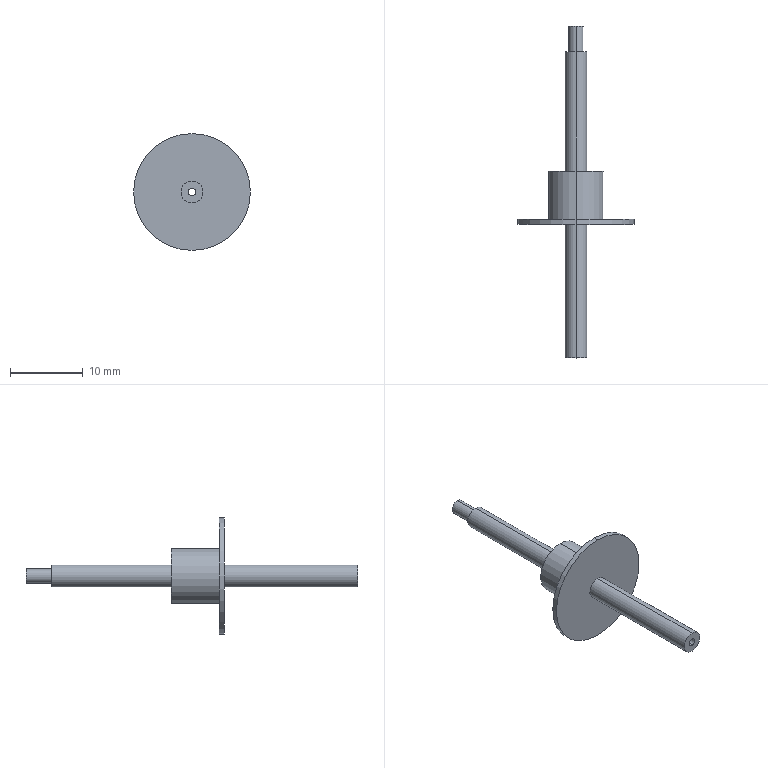Part | SolidWorks | features ICE 2, Revolution 1 | 1 solid | 18 faces | box 16 x 45.5 x 16 mm | volume 652.862 mm3 | cylinder 12 | plane 6 | commonest cylinder face diameters 3 x4 1 x2 2 x2 7.5 x2 16 x2
STEP:
#1=CARTESIAN_POINT('',(0.,42.,1.));
#2=VERTEX_POINT('',#1);
#3=CARTESIAN_POINT('',(0.,42.,-1.));
#4=VERTEX_POINT('',#3);
#5=CARTESIAN_POINT('',(0.,42.,0.));
#6=DIRECTION('',(0.,1.,0.));
#7=DIRECTION('',(0.,0.,1.));
#8=AXIS2_PLACEMENT_3D('',#5,#6,#7);
#9=CIRCLE('',#8,1.);
#10=EDGE_CURVE('',#2,#4,#9,.T.);
#11=ORIENTED_EDGE('',*,*,#10,.T.);
#12=CARTESIAN_POINT('',(0.,45.5,-1.));
#13=VERTEX_POINT('',#12);
#14=CARTESIAN_POINT('',(0.,42.,-1.));
#15=DIRECTION('',(0.,1.,0.));
#16=VECTOR('',#15,1000.);
#17=LINE('',#14,#16);
#18=EDGE_CURVE('',#4,#13,#17,.T.);
#19=ORIENTED_EDGE('',*,*,#18,.T.);
#20=CARTESIAN_POINT('',(0.,45.5,1.));
#21=VERTEX_POINT('',#20);
#22=CARTESIAN_POINT('',(0.,45.5,0.));
#23=DIRECTION('',(0.,1.,0.));
#24=DIRECTION('',(0.,0.,1.));
#25=AXIS2_PLACEMENT_3D('',#22,#23,#24);
#26=CIRCLE('',#25,1.);
#27=EDGE_CURVE('',#21,#13,#26,.T.);
#28=ORIENTED_EDGE('',*,*,#27,.F.);
#29=CARTESIAN_POINT('',(0.,42.,1.));
#30=DIRECTION('',(0.,1.,0.));
#31=VECTOR('',#30,1000.);
#32=LINE('',#29,#31);
#33=EDGE_CURVE('',#2,#21,#32,.T.);
#34=ORIENTED_EDGE('',*,*,#33,.F.);
#35=EDGE_LOOP('',(#11,#19,#28,#34));
#36=FACE_OUTER_BOUND('',#35,.T.);
#37=CARTESIAN_POINT('',(0.,42.,0.));
#38=DIRECTION('',(0.,1.,0.));
#39=DIRECTION('',(0.,0.,1.));
#40=AXIS2_PLACEMENT_3D('',#37,#38,#39);
#41=CYLINDRICAL_SURFACE('',#40,1.);
#42=ADVANCED_FACE('',(#36),#41,.T.);
#43=CARTESIAN_POINT('',(0.,45.5,0.5));
#44=VERTEX_POINT('',#43);
#45=CARTESIAN_POINT('',(0.,45.5,-0.5));
#46=VERTEX_POINT('',#45);
#47=CARTESIAN_POINT('',(0.,45.5,0.));
#48=DIRECTION('',(0.,-1.,0.));
#49=DIRECTION('',(0.,0.,-1.));
#50=AXIS2_PLACEMENT_3D('',#47,#48,#49);
#51=CIRCLE('',#50,0.5);
#52=EDGE_CURVE('',#44,#46,#51,.T.);
#53=ORIENTED_EDGE('',*,*,#52,.F.);
#54=CARTESIAN_POINT('',(0.,0.,0.5));
#55=VERTEX_POINT('',#54);
#56=CARTESIAN_POINT('',(0.,45.5,0.5));
#57=DIRECTION('',(0.,-1.,0.));
#58=VECTOR('',#57,1000.);
#59=LINE('',#56,#58);
#60=EDGE_CURVE('',#44,#55,#59,.T.);
#61=ORIENTED_EDGE('',*,*,#60,.T.);
#62=CARTESIAN_POINT('',(0.,0.,-0.5));
#63=VERTEX_POINT('',#62);
#64=CARTESIAN_POINT('',(0.,0.,0.));
#65=DIRECTION('',(0.,-1.,0.));
#66=DIRECTION('',(0.,0.,-1.));
#67=AXIS2_PLACEMENT_3D('',#64,#65,#66);
#68=CIRCLE('',#67,0.5);
#69=EDGE_CURVE('',#55,#63,#68,.T.);
#70=ORIENTED_EDGE('',*,*,#69,.T.);
#71=CARTESIAN_POINT('',(0.,45.5,-0.5));
#72=DIRECTION('',(0.,-1.,0.));
#73=VECTOR('',#72,1000.);
#74=LINE('',#71,#73);
#75=EDGE_CURVE('',#46,#63,#74,.T.);
#76=ORIENTED_EDGE('',*,*,#75,.F.);
#77=EDGE_LOOP('',(#53,#61,#70,#76));
#78=FACE_OUTER_BOUND('',#77,.T.);
#79=CARTESIAN_POINT('',(0.,45.5,0.));
#80=DIRECTION('',(0.,-1.,0.));
#81=DIRECTION('',(0.,0.,-1.));
#82=AXIS2_PLACEMENT_3D('',#79,#80,#81);
#83=CYLINDRICAL_SURFACE('',#82,0.5);
#84=ADVANCED_FACE('',(#78),#83,.F.);
#85=CARTESIAN_POINT('',(0.,25.6,-3.75));
#86=VERTEX_POINT('',#85);
#87=CARTESIAN_POINT('',(0.,25.6,3.75));
#88=VERTEX_POINT('',#87);
#89=CARTESIAN_POINT('',(0.,25.6,0.));
#90=DIRECTION('',(0.,-1.,0.));
#91=DIRECTION('',(0.,0.,-1.));
#92=AXIS2_PLACEMENT_3D('',#89,#90,#91);
#93=CIRCLE('',#92,3.75);
#94=EDGE_CURVE('',#86,#88,#93,.T.);
#95=ORIENTED_EDGE('',*,*,#94,.T.);
#96=CARTESIAN_POINT('',(0.,19.,3.75));
#97=VERTEX_POINT('',#96);
#98=CARTESIAN_POINT('',(0.,0.,3.75));
#99=DIRECTION('',(0.,-1.,0.));
#100=VECTOR('',#99,1000.);
#101=LINE('',#98,#100);
#102=EDGE_CURVE('',#88,#97,#101,.T.);
#103=ORIENTED_EDGE('',*,*,#102,.T.);
#104=CARTESIAN_POINT('',(0.,19.,-3.75));
#105=VERTEX_POINT('',#104);
#106=CARTESIAN_POINT('',(0.,19.,0.));
#107=DIRECTION('',(0.,-1.,0.));
#108=DIRECTION('',(0.,0.,-1.));
#109=AXIS2_PLACEMENT_3D('',#106,#107,#108);
#110=CIRCLE('',#109,3.75);
#111=EDGE_CURVE('',#105,#97,#110,.T.);
#112=ORIENTED_EDGE('',*,*,#111,.F.);
#113=CARTESIAN_POINT('',(0.,0.,-3.75));
#114=DIRECTION('',(0.,-1.,0.));
#115=VECTOR('',#114,1000.);
#116=LINE('',#113,#115);
#117=EDGE_CURVE('',#86,#105,#116,.T.);
#118=ORIENTED_EDGE('',*,*,#117,.F.);
#119=EDGE_LOOP('',(#95,#103,#112,#118));
#120=FACE_OUTER_BOUND('',#119,.T.);
#121=CARTESIAN_POINT('',(0.,0.,0.));
#122=DIRECTION('',(0.,-1.,0.));
#123=DIRECTION('',(0.,0.,-1.));
#124=AXIS2_PLACEMENT_3D('',#121,#122,#123);
#125=CYLINDRICAL_SURFACE('',#124,3.75);
#126=ADVANCED_FACE('',(#120),#125,.T.);
#127=CARTESIAN_POINT('',(0.,19.,-8.));
#128=VERTEX_POINT('',#127);
#129=CARTESIAN_POINT('',(0.,19.,8.));
#130=VERTEX_POINT('',#129);
#131=CARTESIAN_POINT('',(0.,19.,0.));
#132=DIRECTION('',(0.,-1.,0.));
#133=DIRECTION('',(0.,0.,-1.));
#134=AXIS2_PLACEMENT_3D('',#131,#132,#133);
#135=CIRCLE('',#134,8.);
#136=EDGE_CURVE('',#128,#130,#135,.T.);
#137=ORIENTED_EDGE('',*,*,#136,.T.);
#138=CARTESIAN_POINT('',(0.,18.3,8.));
#139=VERTEX_POINT('',#138);
#140=CARTESIAN_POINT('',(0.,0.,8.));
#141=DIRECTION('',(0.,-1.,0.));
#142=VECTOR('',#141,1000.);
#143=LINE('',#140,#142);
#144=EDGE_CURVE('',#130,#139,#143,.T.);
#145=ORIENTED_EDGE('',*,*,#144,.T.);
#146=CARTESIAN_POINT('',(0.,18.3,-8.));
#147=VERTEX_POINT('',#146);
#148=CARTESIAN_POINT('',(0.,18.3,0.));
#149=DIRECTION('',(0.,-1.,0.));
#150=DIRECTION('',(0.,0.,-1.));
#151=AXIS2_PLACEMENT_3D('',#148,#149,#150);
#152=CIRCLE('',#151,8.);
#153=EDGE_CURVE('',#147,#139,#152,.T.);
#154=ORIENTED_EDGE('',*,*,#153,.F.);
#155=CARTESIAN_POINT('',(0.,0.,-8.));
#156=DIRECTION('',(0.,-1.,0.));
#157=VECTOR('',#156,1000.);
#158=LINE('',#155,#157);
#159=EDGE_CURVE('',#128,#147,#158,.T.);
#160=ORIENTED_EDGE('',*,*,#159,.F.);
#161=EDGE_LOOP('',(#137,#145,#154,#160));
#162=FACE_OUTER_BOUND('',#161,.T.);
#163=CARTESIAN_POINT('',(0.,0.,0.));
#164=DIRECTION('',(0.,-1.,0.));
#165=DIRECTION('',(0.,0.,-1.));
#166=AXIS2_PLACEMENT_3D('',#163,#164,#165);
#167=CYLINDRICAL_SURFACE('',#166,8.);
#168=ADVANCED_FACE('',(#162),#167,.T.);
#169=CARTESIAN_POINT('',(0.,18.3,-1.5));
#170=VERTEX_POINT('',#169);
#171=CARTESIAN_POINT('',(0.,18.3,1.5));
#172=VERTEX_POINT('',#171);
#173=CARTESIAN_POINT('',(0.,18.3,0.));
#174=DIRECTION('',(0.,-1.,0.));
#175=DIRECTION('',(0.,0.,-1.));
#176=AXIS2_PLACEMENT_3D('',#173,#174,#175);
#177=CIRCLE('',#176,1.5);
#178=EDGE_CURVE('',#170,#172,#177,.T.);
#179=ORIENTED_EDGE('',*,*,#178,.T.);
#180=CARTESIAN_POINT('',(0.,0.,1.5));
#181=VERTEX_POINT('',#180);
#182=CARTESIAN_POINT('',(0.,0.,1.5));
#183=DIRECTION('',(0.,-1.,0.));
#184=VECTOR('',#183,1000.);
#185=LINE('',#182,#184);
#186=EDGE_CURVE('',#172,#181,#185,.T.);
#187=ORIENTED_EDGE('',*,*,#186,.T.);
#188=CARTESIAN_POINT('',(0.,0.,-1.5));
#189=VERTEX_POINT('',#188);
#190=CARTESIAN_POINT('',(0.,0.,0.));
#191=DIRECTION('',(0.,-1.,0.));
#192=DIRECTION('',(0.,0.,-1.));
#193=AXIS2_PLACEMENT_3D('',#190,#191,#192);
#194=CIRCLE('',#193,1.5);
#195=EDGE_CURVE('',#189,#181,#194,.T.);
#196=ORIENTED_EDGE('',*,*,#195,.F.);
#197=CARTESIAN_POINT('',(0.,0.,-1.5));
#198=DIRECTION('',(0.,-1.,0.));
#199=VECTOR('',#198,1000.);
#200=LINE('',#197,#199);
#201=EDGE_CURVE('',#170,#189,#200,.T.);
#202=ORIENTED_EDGE('',*,*,#201,.F.);
#203=EDGE_LOOP('',(#179,#187,#196,#202));
#204=FACE_OUTER_BOUND('',#203,.T.);
#205=CARTESIAN_POINT('',(0.,0.,0.));
#206=DIRECTION('',(0.,-1.,0.));
#207=DIRECTION('',(0.,0.,-1.));
#208=AXIS2_PLACEMENT_3D('',#205,#206,#207);
#209=CYLINDRICAL_SURFACE('',#208,1.5);
#210=ADVANCED_FACE('',(#204),#209,.T.);
#211=CARTESIAN_POINT('',(0.,42.,-1.5));
#212=VERTEX_POINT('',#211);
#213=CARTESIAN_POINT('',(0.,42.,1.5));
#214=VERTEX_POINT('',#213);
#215=CARTESIAN_POINT('',(0.,42.,0.));
#216=DIRECTION('',(0.,-1.,0.));
#217=DIRECTION('',(0.,0.,1.));
#218=AXIS2_PLACEMENT_3D('',#215,#216,#217);
#219=CIRCLE('',#218,1.5);
#220=EDGE_CURVE('',#212,#214,#219,.T.);
#221=ORIENTED_EDGE('',*,*,#220,.T.);
#222=CARTESIAN_POINT('',(0.,25.6,1.5));
#223=VERTEX_POINT('',#222);
#224=CARTESIAN_POINT('',(0.,0.,1.5));
#225=DIRECTION('',(0.,-1.,0.));
#226=VECTOR('',#225,1000.);
#227=LINE('',#224,#226);
#228=EDGE_CURVE('',#214,#223,#227,.T.);
#229=ORIENTED_EDGE('',*,*,#228,.T.);
#230=CARTESIAN_POINT('',(0.,25.6,-1.5));
#231=VERTEX_POINT('',#230);
#232=CARTESIAN_POINT('',(0.,25.6,0.));
#233=DIRECTION('',(0.,-1.,0.));
#234=DIRECTION('',(0.,0.,-1.));
#235=AXIS2_PLACEMENT_3D('',#232,#233,#234);
#236=CIRCLE('',#235,1.5);
#237=EDGE_CURVE('',#231,#223,#236,.T.);
#238=ORIENTED_EDGE('',*,*,#237,.F.);
#239=CARTESIAN_POINT('',(0.,0.,-1.5));
#240=DIRECTION('',(0.,-1.,0.));
#241=VECTOR('',#240,1000.);
#242=LINE('',#239,#241);
#243=EDGE_CURVE('',#212,#231,#242,.T.);
#244=ORIENTED_EDGE('',*,*,#243,.F.);
#245=EDGE_LOOP('',(#221,#229,#238,#244));
#246=FACE_OUTER_BOUND('',#245,.T.);
#247=CARTESIAN_POINT('',(0.,0.,0.));
#248=DIRECTION('',(0.,-1.,0.));
#249=DIRECTION('',(0.,0.,-1.));
#250=AXIS2_PLACEMENT_3D('',#247,#248,#249);
#251=CYLINDRICAL_SURFACE('',#250,1.5);
#252=ADVANCED_FACE('',(#246),#251,.T.);
#253=ORIENTED_EDGE('',*,*,#228,.F.);
#254=CARTESIAN_POINT('',(0.,42.,0.));
#255=DIRECTION('',(0.,-1.,0.));
#256=DIRECTION('',(0.,0.,1.));
#257=AXIS2_PLACEMENT_3D('',#254,#255,#256);
#258=CIRCLE('',#257,1.5);
#259=EDGE_CURVE('',#214,#212,#258,.T.);
#260=ORIENTED_EDGE('',*,*,#259,.T.);
#261=ORIENTED_EDGE('',*,*,#243,.T.);
#262=CARTESIAN_POINT('',(0.,25.6,0.));
#263=DIRECTION('',(0.,-1.,0.));
#264=DIRECTION('',(0.,0.,-1.));
#265=AXIS2_PLACEMENT_3D('',#262,#263,#264);
#266=CIRCLE('',#265,1.5);
#267=EDGE_CURVE('',#223,#231,#266,.T.);
#268=ORIENTED_EDGE('',*,*,#267,.F.);
#269=EDGE_LOOP('',(#253,#260,#261,#268));
#270=FACE_OUTER_BOUND('',#269,.T.);
#271=CARTESIAN_POINT('',(0.,0.,0.));
#272=DIRECTION('',(0.,-1.,0.));
#273=DIRECTION('',(0.,0.,-1.));
#274=AXIS2_PLACEMENT_3D('',#271,#272,#273);
#275=CYLINDRICAL_SURFACE('',#274,1.5);
#276=ADVANCED_FACE('',(#270),#275,.T.);
#277=CARTESIAN_POINT('',(0.,45.5,0.));
#278=DIRECTION('',(0.,-1.,0.));
#279=DIRECTION('',(0.,0.,-1.));
#280=AXIS2_PLACEMENT_3D('',#277,#278,#279);
#281=CIRCLE('',#280,0.5);
#282=EDGE_CURVE('',#46,#44,#281,.T.);
#283=ORIENTED_EDGE('',*,*,#282,.T.);
#284=ORIENTED_EDGE('',*,*,#52,.T.);
#285=EDGE_LOOP('',(#283,#284));
#286=FACE_BOUND('',#285,.T.);
#287=ORIENTED_EDGE('',*,*,#27,.T.);
#288=CARTESIAN_POINT('',(0.,45.5,0.));
#289=DIRECTION('',(0.,1.,0.));
#290=DIRECTION('',(0.,0.,1.));
#291=AXIS2_PLACEMENT_3D('',#288,#289,#290);
#292=CIRCLE('',#291,1.);
#293=EDGE_CURVE('',#13,#21,#292,.T.);
#294=ORIENTED_EDGE('',*,*,#293,.T.);
#295=EDGE_LOOP('',(#287,#294));
#296=FACE_OUTER_BOUND('',#295,.T.);
#297=CARTESIAN_POINT('',(1.5,45.5,0.));
#298=DIRECTION('',(0.,1.,0.));
#299=DIRECTION('',(0.,0.,1.));
#300=AXIS2_PLACEMENT_3D('',#297,#298,#299);
#301=PLANE('',#300);
#302=ADVANCED_FACE('',(#286,#296),#301,.T.);
#303=CARTESIAN_POINT('',(0.,0.,0.));
#304=DIRECTION('',(0.,-1.,0.));
#305=DIRECTION('',(0.,0.,-1.));
#306=AXIS2_PLACEMENT_3D('',#303,#304,#305);
#307=CIRCLE('',#306,0.5);
#308=EDGE_CURVE('',#63,#55,#307,.T.);
#309=ORIENTED_EDGE('',*,*,#308,.F.);
#310=ORIENTED_EDGE('',*,*,#69,.F.);
#311=EDGE_LOOP('',(#309,#310));
#312=FACE_BOUND('',#311,.T.);
#313=ORIENTED_EDGE('',*,*,#195,.T.);
#314=CARTESIAN_POINT('',(0.,0.,0.));
#315=DIRECTION('',(0.,-1.,0.));
#316=DIRECTION('',(0.,0.,-1.));
#317=AXIS2_PLACEMENT_3D('',#314,#315,#316);
#318=CIRCLE('',#317,1.5);
#319=EDGE_CURVE('',#181,#189,#318,.T.);
#320=ORIENTED_EDGE('',*,*,#319,.T.);
#321=EDGE_LOOP('',(#313,#320));
#322=FACE_OUTER_BOUND('',#321,.T.);
#323=CARTESIAN_POINT('',(0.,0.,0.));
#324=DIRECTION('',(0.,-1.,0.));
#325=DIRECTION('',(0.,0.,-1.));
#326=AXIS2_PLACEMENT_3D('',#323,#324,#325);
#327=PLANE('',#326);
#328=ADVANCED_FACE('',(#312,#322),#327,.T.);
#329=ORIENTED_EDGE('',*,*,#186,.F.);
#330=CARTESIAN_POINT('',(0.,18.3,0.));
#331=DIRECTION('',(0.,-1.,0.));
#332=DIRECTION('',(0.,0.,-1.));
#333=AXIS2_PLACEMENT_3D('',#330,#331,#332);
#334=CIRCLE('',#333,1.5);
#335=EDGE_CURVE('',#172,#170,#334,.T.);
#336=ORIENTED_EDGE('',*,*,#335,.T.);
#337=ORIENTED_EDGE('',*,*,#201,.T.);
#338=ORIENTED_EDGE('',*,*,#319,.F.);
#339=EDGE_LOOP('',(#329,#336,#337,#338));
#340=FACE_OUTER_BOUND('',#339,.T.);
#341=CARTESIAN_POINT('',(0.,0.,0.));
#342=DIRECTION('',(0.,-1.,0.));
#343=DIRECTION('',(0.,0.,-1.));
#344=AXIS2_PLACEMENT_3D('',#341,#342,#343);
#345=CYLINDRICAL_SURFACE('',#344,1.5);
#346=ADVANCED_FACE('',(#340),#345,.T.);
#347=ORIENTED_EDGE('',*,*,#153,.T.);
#348=CARTESIAN_POINT('',(0.,18.3,0.));
#349=DIRECTION('',(0.,-1.,0.));
#350=DIRECTION('',(0.,0.,-1.));
#351=AXIS2_PLACEMENT_3D('',#348,#349,#350);
#352=CIRCLE('',#351,8.);
#353=EDGE_CURVE('',#139,#147,#352,.T.);
#354=ORIENTED_EDGE('',*,*,#353,.T.);
#355=EDGE_LOOP('',(#347,#354));
#356=FACE_OUTER_BOUND('',#355,.T.);
#357=ORIENTED_EDGE('',*,*,#178,.F.);
#358=ORIENTED_EDGE('',*,*,#335,.F.);
#359=EDGE_LOOP('',(#357,#358));
#360=FACE_BOUND('',#359,.T.);
#361=CARTESIAN_POINT('',(1.5,18.3,0.));
#362=DIRECTION('',(0.,-1.,0.));
#363=DIRECTION('',(0.,0.,-1.));
#364=AXIS2_PLACEMENT_3D('',#361,#362,#363);
#365=PLANE('',#364);
#366=ADVANCED_FACE('',(#356,#360),#365,.T.);
#367=ORIENTED_EDGE('',*,*,#144,.F.);
#368=CARTESIAN_POINT('',(0.,19.,0.));
#369=DIRECTION('',(0.,-1.,0.));
#370=DIRECTION('',(0.,0.,-1.));
#371=AXIS2_PLACEMENT_3D('',#368,#369,#370);
#372=CIRCLE('',#371,8.);
#373=EDGE_CURVE('',#130,#128,#372,.T.);
#374=ORIENTED_EDGE('',*,*,#373,.T.);
#375=ORIENTED_EDGE('',*,*,#159,.T.);
#376=ORIENTED_EDGE('',*,*,#353,.F.);
#377=EDGE_LOOP('',(#367,#374,#375,#376));
#378=FACE_OUTER_BOUND('',#377,.T.);
#379=CARTESIAN_POINT('',(0.,0.,0.));
#380=DIRECTION('',(0.,-1.,0.));
#381=DIRECTION('',(0.,0.,-1.));
#382=AXIS2_PLACEMENT_3D('',#379,#380,#381);
#383=CYLINDRICAL_SURFACE('',#382,8.);
#384=ADVANCED_FACE('',(#378),#383,.T.);
#385=ORIENTED_EDGE('',*,*,#111,.T.);
#386=CARTESIAN_POINT('',(0.,19.,0.));
#387=DIRECTION('',(0.,-1.,0.));
#388=DIRECTION('',(0.,0.,-1.));
#389=AXIS2_PLACEMENT_3D('',#386,#387,#388);
#390=CIRCLE('',#389,3.75);
#391=EDGE_CURVE('',#97,#105,#390,.T.);
#392=ORIENTED_EDGE('',*,*,#391,.T.);
#393=EDGE_LOOP('',(#385,#392));
#394=FACE_BOUND('',#393,.T.);
#395=ORIENTED_EDGE('',*,*,#136,.F.);
#396=ORIENTED_EDGE('',*,*,#373,.F.);
#397=EDGE_LOOP('',(#395,#396));
#398=FACE_OUTER_BOUND('',#397,.T.);
#399=CARTESIAN_POINT('',(8.,19.,0.));
#400=DIRECTION('',(0.,1.,0.));
#401=DIRECTION('',(0.,0.,1.));
#402=AXIS2_PLACEMENT_3D('',#399,#400,#401);
#403=PLANE('',#402);
#404=ADVANCED_FACE('',(#394,#398),#403,.T.);
#405=ORIENTED_EDGE('',*,*,#102,.F.);
#406=CARTESIAN_POINT('',(0.,25.6,0.));
#407=DIRECTION('',(0.,-1.,0.));
#408=DIRECTION('',(0.,0.,-1.));
#409=AXIS2_PLACEMENT_3D('',#406,#407,#408);
#410=CIRCLE('',#409,3.75);
#411=EDGE_CURVE('',#88,#86,#410,.T.);
#412=ORIENTED_EDGE('',*,*,#411,.T.);
#413=ORIENTED_EDGE('',*,*,#117,.T.);
#414=ORIENTED_EDGE('',*,*,#391,.F.);
#415=EDGE_LOOP('',(#405,#412,#413,#414));
#416=FACE_OUTER_BOUND('',#415,.T.);
#417=CARTESIAN_POINT('',(0.,0.,0.));
#418=DIRECTION('',(0.,-1.,0.));
#419=DIRECTION('',(0.,0.,-1.));
#420=AXIS2_PLACEMENT_3D('',#417,#418,#419);
#421=CYLINDRICAL_SURFACE('',#420,3.75);
#422=ADVANCED_FACE('',(#416),#421,.T.);
#423=ORIENTED_EDGE('',*,*,#237,.T.);
#424=ORIENTED_EDGE('',*,*,#267,.T.);
#425=EDGE_LOOP('',(#423,#424));
#426=FACE_BOUND('',#425,.T.);
#427=ORIENTED_EDGE('',*,*,#94,.F.);
#428=ORIENTED_EDGE('',*,*,#411,.F.);
#429=EDGE_LOOP('',(#427,#428));
#430=FACE_OUTER_BOUND('',#429,.T.);
#431=CARTESIAN_POINT('',(3.75,25.6,0.));
#432=DIRECTION('',(0.,1.,0.));
#433=DIRECTION('',(0.,0.,1.));
#434=AXIS2_PLACEMENT_3D('',#431,#432,#433);
#435=PLANE('',#434);
#436=ADVANCED_FACE('',(#426,#430),#435,.T.);
#437=ORIENTED_EDGE('',*,*,#60,.F.);
#438=ORIENTED_EDGE('',*,*,#282,.F.);
#439=ORIENTED_EDGE('',*,*,#75,.T.);
#440=ORIENTED_EDGE('',*,*,#308,.T.);
#441=EDGE_LOOP('',(#437,#438,#439,#440));
#442=FACE_OUTER_BOUND('',#441,.T.);
#443=CARTESIAN_POINT('',(0.,45.5,0.));
#444=DIRECTION('',(0.,-1.,0.));
#445=DIRECTION('',(0.,0.,-1.));
#446=AXIS2_PLACEMENT_3D('',#443,#444,#445);
#447=CYLINDRICAL_SURFACE('',#446,0.5);
#448=ADVANCED_FACE('',(#442),#447,.F.);
#449=ORIENTED_EDGE('',*,*,#220,.F.);
#450=ORIENTED_EDGE('',*,*,#259,.F.);
#451=EDGE_LOOP('',(#449,#450));
#452=FACE_OUTER_BOUND('',#451,.T.);
#453=ORIENTED_EDGE('',*,*,#10,.F.);
#454=CARTESIAN_POINT('',(0.,42.,0.));
#455=DIRECTION('',(0.,1.,0.));
#456=DIRECTION('',(0.,0.,1.));
#457=AXIS2_PLACEMENT_3D('',#454,#455,#456);
#458=CIRCLE('',#457,1.);
#459=EDGE_CURVE('',#4,#2,#458,.T.);
#460=ORIENTED_EDGE('',*,*,#459,.F.);
#461=EDGE_LOOP('',(#453,#460));
#462=FACE_BOUND('',#461,.T.);
#463=CARTESIAN_POINT('',(0.,42.,0.));
#464=DIRECTION('',(0.,1.,0.));
#465=DIRECTION('',(0.,0.,1.));
#466=AXIS2_PLACEMENT_3D('',#463,#464,#465);
#467=PLANE('',#466);
#468=ADVANCED_FACE('',(#452,#462),#467,.T.);
#469=ORIENTED_EDGE('',*,*,#18,.F.);
#470=ORIENTED_EDGE('',*,*,#459,.T.);
#471=ORIENTED_EDGE('',*,*,#33,.T.);
#472=ORIENTED_EDGE('',*,*,#293,.F.);
#473=EDGE_LOOP('',(#469,#470,#471,#472));
#474=FACE_OUTER_BOUND('',#473,.T.);
#475=CARTESIAN_POINT('',(0.,42.,0.));
#476=DIRECTION('',(0.,1.,0.));
#477=DIRECTION('',(0.,0.,1.));
#478=AXIS2_PLACEMENT_3D('',#475,#476,#477);
#479=CYLINDRICAL_SURFACE('',#478,1.);
#480=ADVANCED_FACE('',(#474),#479,.T.);
#481=CLOSED_SHELL('',(#42,#84,#126,#168,#210,#252,#276,#302,#328,#346,#366,#384,#404,#422,#436,#448,#468,#480));
#482=MANIFOLD_SOLID_BREP('',#481);
#483=CARTESIAN_POINT('',(0.,0.,0.));
#484=DIRECTION('',(0.,0.,1.));
#485=DIRECTION('',(1.,0.,0.));
#486=AXIS2_PLACEMENT_3D('',#483,#484,#485);
#487=(LENGTH_UNIT()NAMED_UNIT(*)SI_UNIT(.MILLI.,.METRE.));
#488=UNCERTAINTY_MEASURE_WITH_UNIT(LENGTH_MEASURE(0.00001),#487,'','');
#489=(NAMED_UNIT(*)PLANE_ANGLE_UNIT()SI_UNIT($,.RADIAN.));
#490=(NAMED_UNIT(*)SI_UNIT($,.STERADIAN.)SOLID_ANGLE_UNIT());
#491=(GEOMETRIC_REPRESENTATION_CONTEXT(3)GLOBAL_UNCERTAINTY_ASSIGNED_CONTEXT((#488))GLOBAL_UNIT_ASSIGNED_CONTEXT((#487,#489,#490))REPRESENTATION_CONTEXT('',''));
#492=ADVANCED_BREP_SHAPE_REPRESENTATION('',(#482,#486),#491);